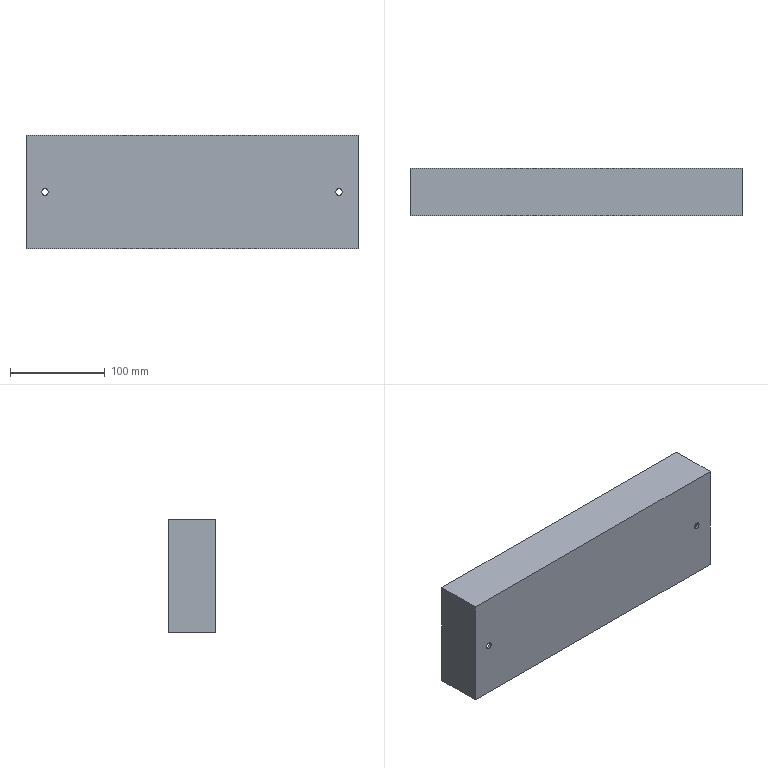Part | STEP file | J451-EBZ05-09-08-Part-1 | 1 solid | 15 faces | box 350 x 50 x 120 mm | volume 185346 mm3 | plane 11 | cylinder 4 | commonest cylinder face diameters 6.8 x4
STEP:
#1=CARTESIAN_POINT('',(0.,0.,0.));
#2=DIRECTION('',(0.,0.,1.));
#3=DIRECTION('',(1.,0.,0.));
#4=AXIS2_PLACEMENT_3D('',#1,#2,#3);
#5=CARTESIAN_POINT('',(16.6,2.3,60.));
#6=VERTEX_POINT('',#5);
#7=CARTESIAN_POINT('',(16.6,0.,60.));
#8=VERTEX_POINT('',#7);
#9=CARTESIAN_POINT('',(16.6,2.3,60.));
#10=DIRECTION('',(0.,-1.,0.));
#11=VECTOR('',#10,1.);
#12=LINE('',#9,#11);
#13=CARTESIAN_POINT('',(20.,2.3,60.));
#14=DIRECTION('',(0.,-1.,0.));
#15=DIRECTION('',(-1.,0.,0.));
#16=AXIS2_PLACEMENT_3D('',#13,#14,#15);
#17=CYLINDRICAL_SURFACE('',#16,3.4);
#18=CARTESIAN_POINT('',(6.283,0.));
#19=DIRECTION('',(0.,1.));
#20=VECTOR('',#19,1.);
#21=LINE('',#18,#20);
#22=(GEOMETRIC_REPRESENTATION_CONTEXT(2)PARAMETRIC_REPRESENTATION_CONTEXT()REPRESENTATION_CONTEXT('',''));
#23=DEFINITIONAL_REPRESENTATION('',(#21),#22);
#24=PCURVE('',#17,#23);
#25=CARTESIAN_POINT('',(20.,2.3,60.));
#26=DIRECTION('',(0.,-1.,0.));
#27=DIRECTION('',(-1.,0.,0.));
#28=AXIS2_PLACEMENT_3D('',#25,#26,#27);
#29=CYLINDRICAL_SURFACE('',#28,3.4);
#30=CARTESIAN_POINT('',(0.,0.));
#31=DIRECTION('',(0.,1.));
#32=VECTOR('',#31,1.);
#33=LINE('',#30,#32);
#34=(GEOMETRIC_REPRESENTATION_CONTEXT(2)PARAMETRIC_REPRESENTATION_CONTEXT()REPRESENTATION_CONTEXT('',''));
#35=DEFINITIONAL_REPRESENTATION('',(#33),#34);
#36=PCURVE('',#29,#35);
#37=SURFACE_CURVE('',#12,(#24,#36),.PCURVE_S1.);
#38=EDGE_CURVE('',#6,#8,#37,.T.);
#39=ORIENTED_EDGE('',*,*,#38,.T.);
#40=CARTESIAN_POINT('',(23.4,0.,60.));
#41=VERTEX_POINT('',#40);
#42=CARTESIAN_POINT('',(20.,0.,60.));
#43=DIRECTION('',(0.,1.,0.));
#44=DIRECTION('',(1.,0.,0.));
#45=AXIS2_PLACEMENT_3D('',#42,#43,#44);
#46=CIRCLE('',#45,3.4);
#47=CARTESIAN_POINT('',(9.425,2.3));
#48=DIRECTION('',(-1.,0.));
#49=VECTOR('',#48,1.);
#50=LINE('',#47,#49);
#51=(GEOMETRIC_REPRESENTATION_CONTEXT(2)PARAMETRIC_REPRESENTATION_CONTEXT()REPRESENTATION_CONTEXT('',''));
#52=DEFINITIONAL_REPRESENTATION('',(#50),#51);
#53=PCURVE('',#17,#52);
#54=CARTESIAN_POINT('',(2.,0.,60.));
#55=DIRECTION('',(0.,-1.,0.));
#56=DIRECTION('',(-1.,0.,0.));
#57=AXIS2_PLACEMENT_3D('',#54,#55,#56);
#58=PLANE('',#57);
#59=CARTESIAN_POINT('',(-21.4,0.));
#60=CARTESIAN_POINT('',(-21.4,5.889));
#61=CARTESIAN_POINT('',(-16.3,2.944));
#62=CARTESIAN_POINT('',(-11.2,0.));
#63=CARTESIAN_POINT('',(-16.3,-2.944));
#64=CARTESIAN_POINT('',(-21.4,-5.889));
#65=CARTESIAN_POINT('',(-21.4,0.));
#66=(BOUNDED_CURVE()B_SPLINE_CURVE(2,(#59,#60,#61,#62,#63,#64,#65),.UNSPECIFIED.,.T.,.F.)B_SPLINE_CURVE_WITH_KNOTS((1,2,2,2,2,1),(-2.094,0.,2.094,4.189,6.283,8.378),.UNSPECIFIED.)CURVE()GEOMETRIC_REPRESENTATION_ITEM()RATIONAL_B_SPLINE_CURVE((1.,0.5,1.,0.5,1.,0.5,1.))REPRESENTATION_ITEM(''));
#67=(GEOMETRIC_REPRESENTATION_CONTEXT(2)PARAMETRIC_REPRESENTATION_CONTEXT()REPRESENTATION_CONTEXT('',''));
#68=DEFINITIONAL_REPRESENTATION('',(#66),#67);
#69=PCURVE('',#58,#68);
#70=SURFACE_CURVE('',#46,(#53,#69),.PCURVE_S1.);
#71=EDGE_CURVE('',#8,#41,#70,.T.);
#72=ORIENTED_EDGE('',*,*,#71,.T.);
#73=CARTESIAN_POINT('',(23.4,2.3,60.));
#74=VERTEX_POINT('',#73);
#75=CARTESIAN_POINT('',(23.4,2.3,60.));
#76=DIRECTION('',(0.,-1.,0.));
#77=VECTOR('',#76,1.);
#78=LINE('',#75,#77);
#79=CARTESIAN_POINT('',(3.142,0.));
#80=DIRECTION('',(0.,1.));
#81=VECTOR('',#80,1.);
#82=LINE('',#79,#81);
#83=(GEOMETRIC_REPRESENTATION_CONTEXT(2)PARAMETRIC_REPRESENTATION_CONTEXT()REPRESENTATION_CONTEXT('',''));
#84=DEFINITIONAL_REPRESENTATION('',(#82),#83);
#85=PCURVE('',#17,#84);
#86=CARTESIAN_POINT('',(3.142,0.));
#87=DIRECTION('',(0.,1.));
#88=VECTOR('',#87,1.);
#89=LINE('',#86,#88);
#90=(GEOMETRIC_REPRESENTATION_CONTEXT(2)PARAMETRIC_REPRESENTATION_CONTEXT()REPRESENTATION_CONTEXT('',''));
#91=DEFINITIONAL_REPRESENTATION('',(#89),#90);
#92=PCURVE('',#29,#91);
#93=SURFACE_CURVE('',#78,(#85,#92),.PCURVE_S1.);
#94=EDGE_CURVE('',#74,#41,#93,.T.);
#95=ORIENTED_EDGE('',*,*,#94,.F.);
#96=CARTESIAN_POINT('',(20.,2.3,60.));
#97=DIRECTION('',(0.,-1.,0.));
#98=DIRECTION('',(-1.,0.,0.));
#99=AXIS2_PLACEMENT_3D('',#96,#97,#98);
#100=CIRCLE('',#99,3.4);
#101=CARTESIAN_POINT('',(0.,0.));
#102=DIRECTION('',(1.,0.));
#103=VECTOR('',#102,1.);
#104=LINE('',#101,#103);
#105=(GEOMETRIC_REPRESENTATION_CONTEXT(2)PARAMETRIC_REPRESENTATION_CONTEXT()REPRESENTATION_CONTEXT('',''));
#106=DEFINITIONAL_REPRESENTATION('',(#104),#105);
#107=PCURVE('',#17,#106);
#108=CARTESIAN_POINT('',(175.,2.3,60.));
#109=DIRECTION('',(0.,1.,0.));
#110=DIRECTION('',(0.,0.,1.));
#111=AXIS2_PLACEMENT_3D('',#108,#109,#110);
#112=PLANE('',#111);
#113=CARTESIAN_POINT('',(0.,-158.4));
#114=CARTESIAN_POINT('',(-5.889,-158.4));
#115=CARTESIAN_POINT('',(-2.944,-153.3));
#116=CARTESIAN_POINT('',(0.,-148.2));
#117=CARTESIAN_POINT('',(2.944,-153.3));
#118=CARTESIAN_POINT('',(5.889,-158.4));
#119=CARTESIAN_POINT('',(0.,-158.4));
#120=(BOUNDED_CURVE()B_SPLINE_CURVE(2,(#113,#114,#115,#116,#117,#118,#119),.UNSPECIFIED.,.T.,.F.)B_SPLINE_CURVE_WITH_KNOTS((1,2,2,2,2,1),(-2.094,0.,2.094,4.189,6.283,8.378),.UNSPECIFIED.)CURVE()GEOMETRIC_REPRESENTATION_ITEM()RATIONAL_B_SPLINE_CURVE((1.,0.5,1.,0.5,1.,0.5,1.))REPRESENTATION_ITEM(''));
#121=(GEOMETRIC_REPRESENTATION_CONTEXT(2)PARAMETRIC_REPRESENTATION_CONTEXT()REPRESENTATION_CONTEXT('',''));
#122=DEFINITIONAL_REPRESENTATION('',(#120),#121);
#123=PCURVE('',#112,#122);
#124=SURFACE_CURVE('',#100,(#107,#123),.PCURVE_S1.);
#125=EDGE_CURVE('',#74,#6,#124,.T.);
#126=ORIENTED_EDGE('',*,*,#125,.T.);
#127=EDGE_LOOP('',(#39,#72,#95,#126));
#128=FACE_BOUND('',#127,.F.);
#129=ADVANCED_FACE('',(#128),#17,.F.);
#130=CARTESIAN_POINT('',(326.6,2.3,60.));
#131=VERTEX_POINT('',#130);
#132=CARTESIAN_POINT('',(326.6,0.,60.));
#133=VERTEX_POINT('',#132);
#134=CARTESIAN_POINT('',(326.6,2.3,60.));
#135=DIRECTION('',(0.,-1.,0.));
#136=VECTOR('',#135,1.);
#137=LINE('',#134,#136);
#138=CARTESIAN_POINT('',(330.,2.3,60.));
#139=DIRECTION('',(0.,-1.,0.));
#140=DIRECTION('',(-1.,0.,0.));
#141=AXIS2_PLACEMENT_3D('',#138,#139,#140);
#142=CYLINDRICAL_SURFACE('',#141,3.4);
#143=CARTESIAN_POINT('',(6.283,0.));
#144=DIRECTION('',(0.,1.));
#145=VECTOR('',#144,1.);
#146=LINE('',#143,#145);
#147=(GEOMETRIC_REPRESENTATION_CONTEXT(2)PARAMETRIC_REPRESENTATION_CONTEXT()REPRESENTATION_CONTEXT('',''));
#148=DEFINITIONAL_REPRESENTATION('',(#146),#147);
#149=PCURVE('',#142,#148);
#150=CARTESIAN_POINT('',(330.,2.3,60.));
#151=DIRECTION('',(0.,-1.,0.));
#152=DIRECTION('',(-1.,0.,0.));
#153=AXIS2_PLACEMENT_3D('',#150,#151,#152);
#154=CYLINDRICAL_SURFACE('',#153,3.4);
#155=CARTESIAN_POINT('',(0.,0.));
#156=DIRECTION('',(0.,1.));
#157=VECTOR('',#156,1.);
#158=LINE('',#155,#157);
#159=(GEOMETRIC_REPRESENTATION_CONTEXT(2)PARAMETRIC_REPRESENTATION_CONTEXT()REPRESENTATION_CONTEXT('',''));
#160=DEFINITIONAL_REPRESENTATION('',(#158),#159);
#161=PCURVE('',#154,#160);
#162=SURFACE_CURVE('',#137,(#149,#161),.PCURVE_S1.);
#163=EDGE_CURVE('',#131,#133,#162,.T.);
#164=ORIENTED_EDGE('',*,*,#163,.T.);
#165=CARTESIAN_POINT('',(333.4,0.,60.));
#166=VERTEX_POINT('',#165);
#167=CARTESIAN_POINT('',(330.,0.,60.));
#168=DIRECTION('',(0.,1.,0.));
#169=DIRECTION('',(1.,0.,0.));
#170=AXIS2_PLACEMENT_3D('',#167,#168,#169);
#171=CIRCLE('',#170,3.4);
#172=CARTESIAN_POINT('',(9.425,2.3));
#173=DIRECTION('',(-1.,0.));
#174=VECTOR('',#173,1.);
#175=LINE('',#172,#174);
#176=(GEOMETRIC_REPRESENTATION_CONTEXT(2)PARAMETRIC_REPRESENTATION_CONTEXT()REPRESENTATION_CONTEXT('',''));
#177=DEFINITIONAL_REPRESENTATION('',(#175),#176);
#178=PCURVE('',#142,#177);
#179=CARTESIAN_POINT('',(-331.4,0.));
#180=CARTESIAN_POINT('',(-331.4,5.889));
#181=CARTESIAN_POINT('',(-326.3,2.944));
#182=CARTESIAN_POINT('',(-321.2,0.));
#183=CARTESIAN_POINT('',(-326.3,-2.944));
#184=CARTESIAN_POINT('',(-331.4,-5.889));
#185=CARTESIAN_POINT('',(-331.4,0.));
#186=(BOUNDED_CURVE()B_SPLINE_CURVE(2,(#179,#180,#181,#182,#183,#184,#185),.UNSPECIFIED.,.T.,.F.)B_SPLINE_CURVE_WITH_KNOTS((1,2,2,2,2,1),(-2.094,0.,2.094,4.189,6.283,8.378),.UNSPECIFIED.)CURVE()GEOMETRIC_REPRESENTATION_ITEM()RATIONAL_B_SPLINE_CURVE((1.,0.5,1.,0.5,1.,0.5,1.))REPRESENTATION_ITEM(''));
#187=(GEOMETRIC_REPRESENTATION_CONTEXT(2)PARAMETRIC_REPRESENTATION_CONTEXT()REPRESENTATION_CONTEXT('',''));
#188=DEFINITIONAL_REPRESENTATION('',(#186),#187);
#189=PCURVE('',#58,#188);
#190=SURFACE_CURVE('',#171,(#178,#189),.PCURVE_S1.);
#191=EDGE_CURVE('',#133,#166,#190,.T.);
#192=ORIENTED_EDGE('',*,*,#191,.T.);
#193=CARTESIAN_POINT('',(333.4,2.3,60.));
#194=VERTEX_POINT('',#193);
#195=CARTESIAN_POINT('',(333.4,2.3,60.));
#196=DIRECTION('',(0.,-1.,0.));
#197=VECTOR('',#196,1.);
#198=LINE('',#195,#197);
#199=CARTESIAN_POINT('',(3.142,0.));
#200=DIRECTION('',(0.,1.));
#201=VECTOR('',#200,1.);
#202=LINE('',#199,#201);
#203=(GEOMETRIC_REPRESENTATION_CONTEXT(2)PARAMETRIC_REPRESENTATION_CONTEXT()REPRESENTATION_CONTEXT('',''));
#204=DEFINITIONAL_REPRESENTATION('',(#202),#203);
#205=PCURVE('',#142,#204);
#206=CARTESIAN_POINT('',(3.142,0.));
#207=DIRECTION('',(0.,1.));
#208=VECTOR('',#207,1.);
#209=LINE('',#206,#208);
#210=(GEOMETRIC_REPRESENTATION_CONTEXT(2)PARAMETRIC_REPRESENTATION_CONTEXT()REPRESENTATION_CONTEXT('',''));
#211=DEFINITIONAL_REPRESENTATION('',(#209),#210);
#212=PCURVE('',#154,#211);
#213=SURFACE_CURVE('',#198,(#205,#212),.PCURVE_S1.);
#214=EDGE_CURVE('',#194,#166,#213,.T.);
#215=ORIENTED_EDGE('',*,*,#214,.F.);
#216=CARTESIAN_POINT('',(330.,2.3,60.));
#217=DIRECTION('',(0.,-1.,0.));
#218=DIRECTION('',(-1.,0.,0.));
#219=AXIS2_PLACEMENT_3D('',#216,#217,#218);
#220=CIRCLE('',#219,3.4);
#221=CARTESIAN_POINT('',(0.,0.));
#222=DIRECTION('',(1.,0.));
#223=VECTOR('',#222,1.);
#224=LINE('',#221,#223);
#225=(GEOMETRIC_REPRESENTATION_CONTEXT(2)PARAMETRIC_REPRESENTATION_CONTEXT()REPRESENTATION_CONTEXT('',''));
#226=DEFINITIONAL_REPRESENTATION('',(#224),#225);
#227=PCURVE('',#142,#226);
#228=CARTESIAN_POINT('',(0.,151.6));
#229=CARTESIAN_POINT('',(-5.889,151.6));
#230=CARTESIAN_POINT('',(-2.944,156.7));
#231=CARTESIAN_POINT('',(0.,161.8));
#232=CARTESIAN_POINT('',(2.944,156.7));
#233=CARTESIAN_POINT('',(5.889,151.6));
#234=CARTESIAN_POINT('',(0.,151.6));
#235=(BOUNDED_CURVE()B_SPLINE_CURVE(2,(#228,#229,#230,#231,#232,#233,#234),.UNSPECIFIED.,.T.,.F.)B_SPLINE_CURVE_WITH_KNOTS((1,2,2,2,2,1),(-2.094,0.,2.094,4.189,6.283,8.378),.UNSPECIFIED.)CURVE()GEOMETRIC_REPRESENTATION_ITEM()RATIONAL_B_SPLINE_CURVE((1.,0.5,1.,0.5,1.,0.5,1.))REPRESENTATION_ITEM(''));
#236=(GEOMETRIC_REPRESENTATION_CONTEXT(2)PARAMETRIC_REPRESENTATION_CONTEXT()REPRESENTATION_CONTEXT('',''));
#237=DEFINITIONAL_REPRESENTATION('',(#235),#236);
#238=PCURVE('',#112,#237);
#239=SURFACE_CURVE('',#220,(#227,#238),.PCURVE_S1.);
#240=EDGE_CURVE('',#194,#131,#239,.T.);
#241=ORIENTED_EDGE('',*,*,#240,.T.);
#242=EDGE_LOOP('',(#164,#192,#215,#241));
#243=FACE_BOUND('',#242,.F.);
#244=ADVANCED_FACE('',(#243),#142,.F.);
#245=CARTESIAN_POINT('',(0.,50.,120.));
#246=VERTEX_POINT('',#245);
#247=CARTESIAN_POINT('',(0.,0.,120.));
#248=VERTEX_POINT('',#247);
#249=CARTESIAN_POINT('',(0.,25.,120.));
#250=DIRECTION('',(0.,-1.,0.));
#251=VECTOR('',#250,1.);
#252=LINE('',#249,#251);
#253=CARTESIAN_POINT('',(0.,25.,60.));
#254=DIRECTION('',(-1.,0.,0.));
#255=DIRECTION('',(0.,1.,0.));
#256=AXIS2_PLACEMENT_3D('',#253,#254,#255);
#257=PLANE('',#256);
#258=CARTESIAN_POINT('',(0.,-60.));
#259=DIRECTION('',(-1.,0.));
#260=VECTOR('',#259,1.);
#261=LINE('',#258,#260);
#262=(GEOMETRIC_REPRESENTATION_CONTEXT(2)PARAMETRIC_REPRESENTATION_CONTEXT()REPRESENTATION_CONTEXT('',''));
#263=DEFINITIONAL_REPRESENTATION('',(#261),#262);
#264=PCURVE('',#257,#263);
#265=CARTESIAN_POINT('',(2.,25.,120.));
#266=DIRECTION('',(0.,0.,1.));
#267=DIRECTION('',(1.,0.,0.));
#268=AXIS2_PLACEMENT_3D('',#265,#266,#267);
#269=PLANE('',#268);
#270=CARTESIAN_POINT('',(-2.,0.));
#271=DIRECTION('',(0.,-1.));
#272=VECTOR('',#271,1.);
#273=LINE('',#270,#272);
#274=(GEOMETRIC_REPRESENTATION_CONTEXT(2)PARAMETRIC_REPRESENTATION_CONTEXT()REPRESENTATION_CONTEXT('',''));
#275=DEFINITIONAL_REPRESENTATION('',(#273),#274);
#276=PCURVE('',#269,#275);
#277=SURFACE_CURVE('',#252,(#264,#276),.PCURVE_S1.);
#278=EDGE_CURVE('',#246,#248,#277,.T.);
#279=ORIENTED_EDGE('',*,*,#278,.F.);
#280=CARTESIAN_POINT('',(0.,50.,0.));
#281=VERTEX_POINT('',#280);
#282=CARTESIAN_POINT('',(0.,50.,60.));
#283=DIRECTION('',(0.,0.,1.));
#284=VECTOR('',#283,1.);
#285=LINE('',#282,#284);
#286=CARTESIAN_POINT('',(25.,0.));
#287=DIRECTION('',(0.,-1.));
#288=VECTOR('',#287,1.);
#289=LINE('',#286,#288);
#290=(GEOMETRIC_REPRESENTATION_CONTEXT(2)PARAMETRIC_REPRESENTATION_CONTEXT()REPRESENTATION_CONTEXT('',''));
#291=DEFINITIONAL_REPRESENTATION('',(#289),#290);
#292=PCURVE('',#257,#291);
#293=CARTESIAN_POINT('',(2.,50.,60.));
#294=DIRECTION('',(0.,1.,0.));
#295=DIRECTION('',(1.,0.,0.));
#296=AXIS2_PLACEMENT_3D('',#293,#294,#295);
#297=PLANE('',#296);
#298=CARTESIAN_POINT('',(-2.,0.));
#299=DIRECTION('',(0.,-1.));
#300=VECTOR('',#299,1.);
#301=LINE('',#298,#300);
#302=(GEOMETRIC_REPRESENTATION_CONTEXT(2)PARAMETRIC_REPRESENTATION_CONTEXT()REPRESENTATION_CONTEXT('',''));
#303=DEFINITIONAL_REPRESENTATION('',(#301),#302);
#304=PCURVE('',#297,#303);
#305=SURFACE_CURVE('',#285,(#292,#304),.PCURVE_S1.);
#306=EDGE_CURVE('',#281,#246,#305,.T.);
#307=ORIENTED_EDGE('',*,*,#306,.F.);
#308=CARTESIAN_POINT('',(0.,0.,0.));
#309=VERTEX_POINT('',#308);
#310=CARTESIAN_POINT('',(0.,25.,0.));
#311=DIRECTION('',(0.,1.,0.));
#312=VECTOR('',#311,1.);
#313=LINE('',#310,#312);
#314=CARTESIAN_POINT('',(0.,60.));
#315=DIRECTION('',(1.,0.));
#316=VECTOR('',#315,1.);
#317=LINE('',#314,#316);
#318=(GEOMETRIC_REPRESENTATION_CONTEXT(2)PARAMETRIC_REPRESENTATION_CONTEXT()REPRESENTATION_CONTEXT('',''));
#319=DEFINITIONAL_REPRESENTATION('',(#317),#318);
#320=PCURVE('',#257,#319);
#321=CARTESIAN_POINT('',(2.,25.,0.));
#322=DIRECTION('',(0.,0.,-1.));
#323=DIRECTION('',(-1.,0.,0.));
#324=AXIS2_PLACEMENT_3D('',#321,#322,#323);
#325=PLANE('',#324);
#326=CARTESIAN_POINT('',(2.,0.));
#327=DIRECTION('',(0.,1.));
#328=VECTOR('',#327,1.);
#329=LINE('',#326,#328);
#330=(GEOMETRIC_REPRESENTATION_CONTEXT(2)PARAMETRIC_REPRESENTATION_CONTEXT()REPRESENTATION_CONTEXT('',''));
#331=DEFINITIONAL_REPRESENTATION('',(#329),#330);
#332=PCURVE('',#325,#331);
#333=SURFACE_CURVE('',#313,(#320,#332),.PCURVE_S1.);
#334=EDGE_CURVE('',#309,#281,#333,.T.);
#335=ORIENTED_EDGE('',*,*,#334,.F.);
#336=CARTESIAN_POINT('',(0.,0.,60.));
#337=DIRECTION('',(0.,0.,-1.));
#338=VECTOR('',#337,1.);
#339=LINE('',#336,#338);
#340=CARTESIAN_POINT('',(-25.,0.));
#341=DIRECTION('',(0.,1.));
#342=VECTOR('',#341,1.);
#343=LINE('',#340,#342);
#344=(GEOMETRIC_REPRESENTATION_CONTEXT(2)PARAMETRIC_REPRESENTATION_CONTEXT()REPRESENTATION_CONTEXT('',''));
#345=DEFINITIONAL_REPRESENTATION('',(#343),#344);
#346=PCURVE('',#257,#345);
#347=CARTESIAN_POINT('',(2.,0.));
#348=DIRECTION('',(0.,1.));
#349=VECTOR('',#348,1.);
#350=LINE('',#347,#349);
#351=(GEOMETRIC_REPRESENTATION_CONTEXT(2)PARAMETRIC_REPRESENTATION_CONTEXT()REPRESENTATION_CONTEXT('',''));
#352=DEFINITIONAL_REPRESENTATION('',(#350),#351);
#353=PCURVE('',#58,#352);
#354=SURFACE_CURVE('',#339,(#346,#353),.PCURVE_S1.);
#355=EDGE_CURVE('',#248,#309,#354,.T.);
#356=ORIENTED_EDGE('',*,*,#355,.F.);
#357=EDGE_LOOP('',(#279,#307,#335,#356));
#358=FACE_BOUND('',#357,.T.);
#359=ADVANCED_FACE('',(#358),#257,.T.);
#360=ORIENTED_EDGE('',*,*,#278,.T.);
#361=CARTESIAN_POINT('',(350.,0.,120.));
#362=VERTEX_POINT('',#361);
#363=CARTESIAN_POINT('',(2.,0.,120.));
#364=DIRECTION('',(-1.,0.,0.));
#365=VECTOR('',#364,1.);
#366=LINE('',#363,#365);
#367=CARTESIAN_POINT('',(0.,-25.));
#368=DIRECTION('',(-1.,0.));
#369=VECTOR('',#368,1.);
#370=LINE('',#367,#369);
#371=(GEOMETRIC_REPRESENTATION_CONTEXT(2)PARAMETRIC_REPRESENTATION_CONTEXT()REPRESENTATION_CONTEXT('',''));
#372=DEFINITIONAL_REPRESENTATION('',(#370),#371);
#373=PCURVE('',#269,#372);
#374=CARTESIAN_POINT('',(0.,-60.));
#375=DIRECTION('',(1.,0.));
#376=VECTOR('',#375,1.);
#377=LINE('',#374,#376);
#378=(GEOMETRIC_REPRESENTATION_CONTEXT(2)PARAMETRIC_REPRESENTATION_CONTEXT()REPRESENTATION_CONTEXT('',''));
#379=DEFINITIONAL_REPRESENTATION('',(#377),#378);
#380=PCURVE('',#58,#379);
#381=SURFACE_CURVE('',#366,(#373,#380),.PCURVE_S1.);
#382=EDGE_CURVE('',#362,#248,#381,.T.);
#383=ORIENTED_EDGE('',*,*,#382,.F.);
#384=CARTESIAN_POINT('',(350.,50.,120.));
#385=VERTEX_POINT('',#384);
#386=CARTESIAN_POINT('',(350.,25.,120.));
#387=DIRECTION('',(0.,-1.,0.));
#388=VECTOR('',#387,1.);
#389=LINE('',#386,#388);
#390=CARTESIAN_POINT('',(348.,0.));
#391=DIRECTION('',(0.,-1.));
#392=VECTOR('',#391,1.);
#393=LINE('',#390,#392);
#394=(GEOMETRIC_REPRESENTATION_CONTEXT(2)PARAMETRIC_REPRESENTATION_CONTEXT()REPRESENTATION_CONTEXT('',''));
#395=DEFINITIONAL_REPRESENTATION('',(#393),#394);
#396=PCURVE('',#269,#395);
#397=CARTESIAN_POINT('',(350.,25.,120.));
#398=DIRECTION('',(1.,0.,0.));
#399=DIRECTION('',(0.,0.,-1.));
#400=AXIS2_PLACEMENT_3D('',#397,#398,#399);
#401=PLANE('',#400);
#402=CARTESIAN_POINT('',(0.,0.));
#403=DIRECTION('',(0.,-1.));
#404=VECTOR('',#403,1.);
#405=LINE('',#402,#404);
#406=(GEOMETRIC_REPRESENTATION_CONTEXT(2)PARAMETRIC_REPRESENTATION_CONTEXT()REPRESENTATION_CONTEXT('',''));
#407=DEFINITIONAL_REPRESENTATION('',(#405),#406);
#408=PCURVE('',#401,#407);
#409=SURFACE_CURVE('',#389,(#396,#408),.PCURVE_S1.);
#410=EDGE_CURVE('',#385,#362,#409,.T.);
#411=ORIENTED_EDGE('',*,*,#410,.F.);
#412=CARTESIAN_POINT('',(2.,50.,120.));
#413=DIRECTION('',(-1.,0.,0.));
#414=VECTOR('',#413,1.);
#415=LINE('',#412,#414);
#416=CARTESIAN_POINT('',(0.,25.));
#417=DIRECTION('',(-1.,0.));
#418=VECTOR('',#417,1.);
#419=LINE('',#416,#418);
#420=(GEOMETRIC_REPRESENTATION_CONTEXT(2)PARAMETRIC_REPRESENTATION_CONTEXT()REPRESENTATION_CONTEXT('',''));
#421=DEFINITIONAL_REPRESENTATION('',(#419),#420);
#422=PCURVE('',#269,#421);
#423=CARTESIAN_POINT('',(0.,-60.));
#424=DIRECTION('',(-1.,0.));
#425=VECTOR('',#424,1.);
#426=LINE('',#423,#425);
#427=(GEOMETRIC_REPRESENTATION_CONTEXT(2)PARAMETRIC_REPRESENTATION_CONTEXT()REPRESENTATION_CONTEXT('',''));
#428=DEFINITIONAL_REPRESENTATION('',(#426),#427);
#429=PCURVE('',#297,#428);
#430=SURFACE_CURVE('',#415,(#422,#429),.PCURVE_S1.);
#431=EDGE_CURVE('',#385,#246,#430,.T.);
#432=ORIENTED_EDGE('',*,*,#431,.T.);
#433=EDGE_LOOP('',(#360,#383,#411,#432));
#434=FACE_BOUND('',#433,.T.);
#435=ADVANCED_FACE('',(#434),#269,.T.);
#436=ORIENTED_EDGE('',*,*,#71,.T.);
#437=CARTESIAN_POINT('',(20.,0.,60.));
#438=DIRECTION('',(0.,1.,0.));
#439=DIRECTION('',(1.,0.,0.));
#440=AXIS2_PLACEMENT_3D('',#437,#438,#439);
#441=CIRCLE('',#440,3.4);
#442=CARTESIAN_POINT('',(-21.4,0.));
#443=CARTESIAN_POINT('',(-21.4,5.889));
#444=CARTESIAN_POINT('',(-16.3,2.944));
#445=CARTESIAN_POINT('',(-11.2,0.));
#446=CARTESIAN_POINT('',(-16.3,-2.944));
#447=CARTESIAN_POINT('',(-21.4,-5.889));
#448=CARTESIAN_POINT('',(-21.4,0.));
#449=(BOUNDED_CURVE()B_SPLINE_CURVE(2,(#442,#443,#444,#445,#446,#447,#448),.UNSPECIFIED.,.T.,.F.)B_SPLINE_CURVE_WITH_KNOTS((1,2,2,2,2,1),(-2.094,0.,2.094,4.189,6.283,8.378),.UNSPECIFIED.)CURVE()GEOMETRIC_REPRESENTATION_ITEM()RATIONAL_B_SPLINE_CURVE((1.,0.5,1.,0.5,1.,0.5,1.))REPRESENTATION_ITEM(''));
#450=(GEOMETRIC_REPRESENTATION_CONTEXT(2)PARAMETRIC_REPRESENTATION_CONTEXT()REPRESENTATION_CONTEXT('',''));
#451=DEFINITIONAL_REPRESENTATION('',(#449),#450);
#452=PCURVE('',#58,#451);
#453=CARTESIAN_POINT('',(3.142,2.3));
#454=DIRECTION('',(-1.,0.));
#455=VECTOR('',#454,1.);
#456=LINE('',#453,#455);
#457=(GEOMETRIC_REPRESENTATION_CONTEXT(2)PARAMETRIC_REPRESENTATION_CONTEXT()REPRESENTATION_CONTEXT('',''));
#458=DEFINITIONAL_REPRESENTATION('',(#456),#457);
#459=PCURVE('',#29,#458);
#460=SURFACE_CURVE('',#441,(#452,#459),.PCURVE_S1.);
#461=EDGE_CURVE('',#41,#8,#460,.T.);
#462=ORIENTED_EDGE('',*,*,#461,.T.);
#463=EDGE_LOOP('',(#436,#462));
#464=FACE_BOUND('',#463,.T.);
#465=ORIENTED_EDGE('',*,*,#191,.T.);
#466=CARTESIAN_POINT('',(330.,0.,60.));
#467=DIRECTION('',(0.,1.,0.));
#468=DIRECTION('',(1.,0.,0.));
#469=AXIS2_PLACEMENT_3D('',#466,#467,#468);
#470=CIRCLE('',#469,3.4);
#471=CARTESIAN_POINT('',(-331.4,0.));
#472=CARTESIAN_POINT('',(-331.4,5.889));
#473=CARTESIAN_POINT('',(-326.3,2.944));
#474=CARTESIAN_POINT('',(-321.2,0.));
#475=CARTESIAN_POINT('',(-326.3,-2.944));
#476=CARTESIAN_POINT('',(-331.4,-5.889));
#477=CARTESIAN_POINT('',(-331.4,0.));
#478=(BOUNDED_CURVE()B_SPLINE_CURVE(2,(#471,#472,#473,#474,#475,#476,#477),.UNSPECIFIED.,.T.,.F.)B_SPLINE_CURVE_WITH_KNOTS((1,2,2,2,2,1),(-2.094,0.,2.094,4.189,6.283,8.378),.UNSPECIFIED.)CURVE()GEOMETRIC_REPRESENTATION_ITEM()RATIONAL_B_SPLINE_CURVE((1.,0.5,1.,0.5,1.,0.5,1.))REPRESENTATION_ITEM(''));
#479=(GEOMETRIC_REPRESENTATION_CONTEXT(2)PARAMETRIC_REPRESENTATION_CONTEXT()REPRESENTATION_CONTEXT('',''));
#480=DEFINITIONAL_REPRESENTATION('',(#478),#479);
#481=PCURVE('',#58,#480);
#482=CARTESIAN_POINT('',(3.142,2.3));
#483=DIRECTION('',(-1.,0.));
#484=VECTOR('',#483,1.);
#485=LINE('',#482,#484);
#486=(GEOMETRIC_REPRESENTATION_CONTEXT(2)PARAMETRIC_REPRESENTATION_CONTEXT()REPRESENTATION_CONTEXT('',''));
#487=DEFINITIONAL_REPRESENTATION('',(#485),#486);
#488=PCURVE('',#154,#487);
#489=SURFACE_CURVE('',#470,(#481,#488),.PCURVE_S1.);
#490=EDGE_CURVE('',#166,#133,#489,.T.);
#491=ORIENTED_EDGE('',*,*,#490,.T.);
#492=EDGE_LOOP('',(#465,#491));
#493=FACE_BOUND('',#492,.T.);
#494=CARTESIAN_POINT('',(350.,0.,0.));
#495=VERTEX_POINT('',#494);
#496=CARTESIAN_POINT('',(2.,0.,0.));
#497=DIRECTION('',(-1.,0.,0.));
#498=VECTOR('',#497,1.);
#499=LINE('',#496,#498);
#500=CARTESIAN_POINT('',(0.,60.));
#501=DIRECTION('',(1.,0.));
#502=VECTOR('',#501,1.);
#503=LINE('',#500,#502);
#504=(GEOMETRIC_REPRESENTATION_CONTEXT(2)PARAMETRIC_REPRESENTATION_CONTEXT()REPRESENTATION_CONTEXT('',''));
#505=DEFINITIONAL_REPRESENTATION('',(#503),#504);
#506=PCURVE('',#58,#505);
#507=CARTESIAN_POINT('',(0.,-25.));
#508=DIRECTION('',(1.,0.));
#509=VECTOR('',#508,1.);
#510=LINE('',#507,#509);
#511=(GEOMETRIC_REPRESENTATION_CONTEXT(2)PARAMETRIC_REPRESENTATION_CONTEXT()REPRESENTATION_CONTEXT('',''));
#512=DEFINITIONAL_REPRESENTATION('',(#510),#511);
#513=PCURVE('',#325,#512);
#514=SURFACE_CURVE('',#499,(#506,#513),.PCURVE_S1.);
#515=EDGE_CURVE('',#495,#309,#514,.T.);
#516=ORIENTED_EDGE('',*,*,#515,.F.);
#517=CARTESIAN_POINT('',(350.,0.,120.));
#518=DIRECTION('',(0.,0.,-1.));
#519=VECTOR('',#518,1.);
#520=LINE('',#517,#519);
#521=CARTESIAN_POINT('',(-348.,-60.));
#522=DIRECTION('',(0.,1.));
#523=VECTOR('',#522,1.);
#524=LINE('',#521,#523);
#525=(GEOMETRIC_REPRESENTATION_CONTEXT(2)PARAMETRIC_REPRESENTATION_CONTEXT()REPRESENTATION_CONTEXT('',''));
#526=DEFINITIONAL_REPRESENTATION('',(#524),#525);
#527=PCURVE('',#58,#526);
#528=CARTESIAN_POINT('',(0.,-25.));
#529=DIRECTION('',(1.,0.));
#530=VECTOR('',#529,1.);
#531=LINE('',#528,#530);
#532=(GEOMETRIC_REPRESENTATION_CONTEXT(2)PARAMETRIC_REPRESENTATION_CONTEXT()REPRESENTATION_CONTEXT('',''));
#533=DEFINITIONAL_REPRESENTATION('',(#531),#532);
#534=PCURVE('',#401,#533);
#535=SURFACE_CURVE('',#520,(#527,#534),.PCURVE_S1.);
#536=EDGE_CURVE('',#362,#495,#535,.T.);
#537=ORIENTED_EDGE('',*,*,#536,.F.);
#538=ORIENTED_EDGE('',*,*,#382,.T.);
#539=ORIENTED_EDGE('',*,*,#355,.T.);
#540=EDGE_LOOP('',(#516,#537,#538,#539));
#541=FACE_BOUND('',#540,.T.);
#542=ADVANCED_FACE('',(#464,#493,#541),#58,.T.);
#543=CARTESIAN_POINT('',(350.,50.,0.));
#544=VERTEX_POINT('',#543);
#545=CARTESIAN_POINT('',(2.,50.,0.));
#546=DIRECTION('',(-1.,0.,0.));
#547=VECTOR('',#546,1.);
#548=LINE('',#545,#547);
#549=CARTESIAN_POINT('',(0.,25.));
#550=DIRECTION('',(1.,0.));
#551=VECTOR('',#550,1.);
#552=LINE('',#549,#551);
#553=(GEOMETRIC_REPRESENTATION_CONTEXT(2)PARAMETRIC_REPRESENTATION_CONTEXT()REPRESENTATION_CONTEXT('',''));
#554=DEFINITIONAL_REPRESENTATION('',(#552),#553);
#555=PCURVE('',#325,#554);
#556=CARTESIAN_POINT('',(0.,60.));
#557=DIRECTION('',(-1.,0.));
#558=VECTOR('',#557,1.);
#559=LINE('',#556,#558);
#560=(GEOMETRIC_REPRESENTATION_CONTEXT(2)PARAMETRIC_REPRESENTATION_CONTEXT()REPRESENTATION_CONTEXT('',''));
#561=DEFINITIONAL_REPRESENTATION('',(#559),#560);
#562=PCURVE('',#297,#561);
#563=SURFACE_CURVE('',#548,(#555,#562),.PCURVE_S1.);
#564=EDGE_CURVE('',#544,#281,#563,.T.);
#565=ORIENTED_EDGE('',*,*,#564,.F.);
#566=CARTESIAN_POINT('',(350.,25.,0.));
#567=DIRECTION('',(0.,-1.,0.));
#568=VECTOR('',#567,1.);
#569=LINE('',#566,#568);
#570=CARTESIAN_POINT('',(-348.,0.));
#571=DIRECTION('',(0.,-1.));
#572=VECTOR('',#571,1.);
#573=LINE('',#570,#572);
#574=(GEOMETRIC_REPRESENTATION_CONTEXT(2)PARAMETRIC_REPRESENTATION_CONTEXT()REPRESENTATION_CONTEXT('',''));
#575=DEFINITIONAL_REPRESENTATION('',(#573),#574);
#576=PCURVE('',#325,#575);
#577=CARTESIAN_POINT('',(120.,0.));
#578=DIRECTION('',(0.,-1.));
#579=VECTOR('',#578,1.);
#580=LINE('',#577,#579);
#581=(GEOMETRIC_REPRESENTATION_CONTEXT(2)PARAMETRIC_REPRESENTATION_CONTEXT()REPRESENTATION_CONTEXT('',''));
#582=DEFINITIONAL_REPRESENTATION('',(#580),#581);
#583=PCURVE('',#401,#582);
#584=SURFACE_CURVE('',#569,(#576,#583),.PCURVE_S1.);
#585=EDGE_CURVE('',#544,#495,#584,.T.);
#586=ORIENTED_EDGE('',*,*,#585,.T.);
#587=ORIENTED_EDGE('',*,*,#515,.T.);
#588=ORIENTED_EDGE('',*,*,#334,.T.);
#589=EDGE_LOOP('',(#565,#586,#587,#588));
#590=FACE_BOUND('',#589,.T.);
#591=ADVANCED_FACE('',(#590),#325,.T.);
#592=CARTESIAN_POINT('',(2.,2.3,118.));
#593=VERTEX_POINT('',#592);
#594=CARTESIAN_POINT('',(2.,50.,118.));
#595=VERTEX_POINT('',#594);
#596=CARTESIAN_POINT('',(2.,25.,118.));
#597=DIRECTION('',(0.,1.,0.));
#598=VECTOR('',#597,1.);
#599=LINE('',#596,#598);
#600=CARTESIAN_POINT('',(2.,25.,60.));
#601=DIRECTION('',(1.,0.,0.));
#602=DIRECTION('',(0.,-1.,0.));
#603=AXIS2_PLACEMENT_3D('',#600,#601,#602);
#604=PLANE('',#603);
#605=CARTESIAN_POINT('',(0.,-58.));
#606=DIRECTION('',(-1.,0.));
#607=VECTOR('',#606,1.);
#608=LINE('',#605,#607);
#609=(GEOMETRIC_REPRESENTATION_CONTEXT(2)PARAMETRIC_REPRESENTATION_CONTEXT()REPRESENTATION_CONTEXT('',''));
#610=DEFINITIONAL_REPRESENTATION('',(#608),#609);
#611=PCURVE('',#604,#610);
#612=CARTESIAN_POINT('',(175.,25.,118.));
#613=DIRECTION('',(0.,0.,-1.));
#614=DIRECTION('',(0.,1.,0.));
#615=AXIS2_PLACEMENT_3D('',#612,#613,#614);
#616=PLANE('',#615);
#617=CARTESIAN_POINT('',(0.,-173.));
#618=DIRECTION('',(1.,0.));
#619=VECTOR('',#618,1.);
#620=LINE('',#617,#619);
#621=(GEOMETRIC_REPRESENTATION_CONTEXT(2)PARAMETRIC_REPRESENTATION_CONTEXT()REPRESENTATION_CONTEXT('',''));
#622=DEFINITIONAL_REPRESENTATION('',(#620),#621);
#623=PCURVE('',#616,#622);
#624=SURFACE_CURVE('',#599,(#611,#623),.PCURVE_S1.);
#625=EDGE_CURVE('',#593,#595,#624,.T.);
#626=ORIENTED_EDGE('',*,*,#625,.F.);
#627=CARTESIAN_POINT('',(2.,2.3,2.));
#628=VERTEX_POINT('',#627);
#629=CARTESIAN_POINT('',(2.,2.3,60.));
#630=DIRECTION('',(0.,0.,1.));
#631=VECTOR('',#630,1.);
#632=LINE('',#629,#631);
#633=CARTESIAN_POINT('',(22.7,0.));
#634=DIRECTION('',(0.,-1.));
#635=VECTOR('',#634,1.);
#636=LINE('',#633,#635);
#637=(GEOMETRIC_REPRESENTATION_CONTEXT(2)PARAMETRIC_REPRESENTATION_CONTEXT()REPRESENTATION_CONTEXT('',''));
#638=DEFINITIONAL_REPRESENTATION('',(#636),#637);
#639=PCURVE('',#604,#638);
#640=CARTESIAN_POINT('',(0.,-173.));
#641=DIRECTION('',(1.,0.));
#642=VECTOR('',#641,1.);
#643=LINE('',#640,#642);
#644=(GEOMETRIC_REPRESENTATION_CONTEXT(2)PARAMETRIC_REPRESENTATION_CONTEXT()REPRESENTATION_CONTEXT('',''));
#645=DEFINITIONAL_REPRESENTATION('',(#643),#644);
#646=PCURVE('',#112,#645);
#647=SURFACE_CURVE('',#632,(#639,#646),.PCURVE_S1.);
#648=EDGE_CURVE('',#628,#593,#647,.T.);
#649=ORIENTED_EDGE('',*,*,#648,.F.);
#650=CARTESIAN_POINT('',(2.,50.,2.));
#651=VERTEX_POINT('',#650);
#652=CARTESIAN_POINT('',(2.,25.,2.));
#653=DIRECTION('',(0.,-1.,0.));
#654=VECTOR('',#653,1.);
#655=LINE('',#652,#654);
#656=CARTESIAN_POINT('',(0.,58.));
#657=DIRECTION('',(1.,0.));
#658=VECTOR('',#657,1.);
#659=LINE('',#656,#658);
#660=(GEOMETRIC_REPRESENTATION_CONTEXT(2)PARAMETRIC_REPRESENTATION_CONTEXT()REPRESENTATION_CONTEXT('',''));
#661=DEFINITIONAL_REPRESENTATION('',(#659),#660);
#662=PCURVE('',#604,#661);
#663=CARTESIAN_POINT('',(175.,25.,2.));
#664=DIRECTION('',(0.,0.,1.));
#665=DIRECTION('',(0.,-1.,0.));
#666=AXIS2_PLACEMENT_3D('',#663,#664,#665);
#667=PLANE('',#666);
#668=CARTESIAN_POINT('',(0.,-173.));
#669=DIRECTION('',(1.,0.));
#670=VECTOR('',#669,1.);
#671=LINE('',#668,#670);
#672=(GEOMETRIC_REPRESENTATION_CONTEXT(2)PARAMETRIC_REPRESENTATION_CONTEXT()REPRESENTATION_CONTEXT('',''));
#673=DEFINITIONAL_REPRESENTATION('',(#671),#672);
#674=PCURVE('',#667,#673);
#675=SURFACE_CURVE('',#655,(#662,#674),.PCURVE_S1.);
#676=EDGE_CURVE('',#651,#628,#675,.T.);
#677=ORIENTED_EDGE('',*,*,#676,.F.);
#678=CARTESIAN_POINT('',(2.,50.,60.));
#679=DIRECTION('',(0.,0.,-1.));
#680=VECTOR('',#679,1.);
#681=LINE('',#678,#680);
#682=CARTESIAN_POINT('',(-25.,0.));
#683=DIRECTION('',(0.,1.));
#684=VECTOR('',#683,1.);
#685=LINE('',#682,#684);
#686=(GEOMETRIC_REPRESENTATION_CONTEXT(2)PARAMETRIC_REPRESENTATION_CONTEXT()REPRESENTATION_CONTEXT('',''));
#687=DEFINITIONAL_REPRESENTATION('',(#685),#686);
#688=PCURVE('',#604,#687);
#689=CARTESIAN_POINT('',(0.,0.));
#690=DIRECTION('',(0.,1.));
#691=VECTOR('',#690,1.);
#692=LINE('',#689,#691);
#693=(GEOMETRIC_REPRESENTATION_CONTEXT(2)PARAMETRIC_REPRESENTATION_CONTEXT()REPRESENTATION_CONTEXT('',''));
#694=DEFINITIONAL_REPRESENTATION('',(#692),#693);
#695=PCURVE('',#297,#694);
#696=SURFACE_CURVE('',#681,(#688,#695),.PCURVE_S1.);
#697=EDGE_CURVE('',#595,#651,#696,.T.);
#698=ORIENTED_EDGE('',*,*,#697,.F.);
#699=EDGE_LOOP('',(#626,#649,#677,#698));
#700=FACE_BOUND('',#699,.T.);
#701=ADVANCED_FACE('',(#700),#604,.T.);
#702=CARTESIAN_POINT('',(348.,50.,2.));
#703=VERTEX_POINT('',#702);
#704=CARTESIAN_POINT('',(175.,50.,2.));
#705=DIRECTION('',(1.,0.,0.));
#706=VECTOR('',#705,1.);
#707=LINE('',#704,#706);
#708=CARTESIAN_POINT('',(173.,58.));
#709=DIRECTION('',(1.,0.));
#710=VECTOR('',#709,1.);
#711=LINE('',#708,#710);
#712=(GEOMETRIC_REPRESENTATION_CONTEXT(2)PARAMETRIC_REPRESENTATION_CONTEXT()REPRESENTATION_CONTEXT('',''));
#713=DEFINITIONAL_REPRESENTATION('',(#711),#712);
#714=PCURVE('',#297,#713);
#715=CARTESIAN_POINT('',(-25.,0.));
#716=DIRECTION('',(0.,1.));
#717=VECTOR('',#716,1.);
#718=LINE('',#715,#717);
#719=(GEOMETRIC_REPRESENTATION_CONTEXT(2)PARAMETRIC_REPRESENTATION_CONTEXT()REPRESENTATION_CONTEXT('',''));
#720=DEFINITIONAL_REPRESENTATION('',(#718),#719);
#721=PCURVE('',#667,#720);
#722=SURFACE_CURVE('',#707,(#714,#721),.PCURVE_S1.);
#723=EDGE_CURVE('',#651,#703,#722,.T.);
#724=ORIENTED_EDGE('',*,*,#723,.T.);
#725=CARTESIAN_POINT('',(348.,50.,118.));
#726=VERTEX_POINT('',#725);
#727=CARTESIAN_POINT('',(348.,50.,60.));
#728=DIRECTION('',(0.,0.,1.));
#729=VECTOR('',#728,1.);
#730=LINE('',#727,#729);
#731=CARTESIAN_POINT('',(346.,0.));
#732=DIRECTION('',(0.,-1.));
#733=VECTOR('',#732,1.);
#734=LINE('',#731,#733);
#735=(GEOMETRIC_REPRESENTATION_CONTEXT(2)PARAMETRIC_REPRESENTATION_CONTEXT()REPRESENTATION_CONTEXT('',''));
#736=DEFINITIONAL_REPRESENTATION('',(#734),#735);
#737=PCURVE('',#297,#736);
#738=CARTESIAN_POINT('',(348.,25.,60.));
#739=DIRECTION('',(-1.,0.,0.));
#740=DIRECTION('',(0.,1.,0.));
#741=AXIS2_PLACEMENT_3D('',#738,#739,#740);
#742=PLANE('',#741);
#743=CARTESIAN_POINT('',(25.,0.));
#744=DIRECTION('',(0.,-1.));
#745=VECTOR('',#744,1.);
#746=LINE('',#743,#745);
#747=(GEOMETRIC_REPRESENTATION_CONTEXT(2)PARAMETRIC_REPRESENTATION_CONTEXT()REPRESENTATION_CONTEXT('',''));
#748=DEFINITIONAL_REPRESENTATION('',(#746),#747);
#749=PCURVE('',#742,#748);
#750=SURFACE_CURVE('',#730,(#737,#749),.PCURVE_S1.);
#751=EDGE_CURVE('',#703,#726,#750,.T.);
#752=ORIENTED_EDGE('',*,*,#751,.T.);
#753=CARTESIAN_POINT('',(175.,50.,118.));
#754=DIRECTION('',(-1.,0.,0.));
#755=VECTOR('',#754,1.);
#756=LINE('',#753,#755);
#757=CARTESIAN_POINT('',(173.,-58.));
#758=DIRECTION('',(-1.,0.));
#759=VECTOR('',#758,1.);
#760=LINE('',#757,#759);
#761=(GEOMETRIC_REPRESENTATION_CONTEXT(2)PARAMETRIC_REPRESENTATION_CONTEXT()REPRESENTATION_CONTEXT('',''));
#762=DEFINITIONAL_REPRESENTATION('',(#760),#761);
#763=PCURVE('',#297,#762);
#764=CARTESIAN_POINT('',(25.,0.));
#765=DIRECTION('',(0.,-1.));
#766=VECTOR('',#765,1.);
#767=LINE('',#764,#766);
#768=(GEOMETRIC_REPRESENTATION_CONTEXT(2)PARAMETRIC_REPRESENTATION_CONTEXT()REPRESENTATION_CONTEXT('',''));
#769=DEFINITIONAL_REPRESENTATION('',(#767),#768);
#770=PCURVE('',#616,#769);
#771=SURFACE_CURVE('',#756,(#763,#770),.PCURVE_S1.);
#772=EDGE_CURVE('',#726,#595,#771,.T.);
#773=ORIENTED_EDGE('',*,*,#772,.T.);
#774=ORIENTED_EDGE('',*,*,#697,.T.);
#775=EDGE_LOOP('',(#724,#752,#773,#774));
#776=FACE_BOUND('',#775,.T.);
#777=ORIENTED_EDGE('',*,*,#306,.T.);
#778=ORIENTED_EDGE('',*,*,#431,.F.);
#779=CARTESIAN_POINT('',(350.,50.,120.));
#780=DIRECTION('',(0.,0.,-1.));
#781=VECTOR('',#780,1.);
#782=LINE('',#779,#781);
#783=CARTESIAN_POINT('',(348.,-60.));
#784=DIRECTION('',(0.,1.));
#785=VECTOR('',#784,1.);
#786=LINE('',#783,#785);
#787=(GEOMETRIC_REPRESENTATION_CONTEXT(2)PARAMETRIC_REPRESENTATION_CONTEXT()REPRESENTATION_CONTEXT('',''));
#788=DEFINITIONAL_REPRESENTATION('',(#786),#787);
#789=PCURVE('',#297,#788);
#790=CARTESIAN_POINT('',(0.,25.));
#791=DIRECTION('',(1.,0.));
#792=VECTOR('',#791,1.);
#793=LINE('',#790,#792);
#794=(GEOMETRIC_REPRESENTATION_CONTEXT(2)PARAMETRIC_REPRESENTATION_CONTEXT()REPRESENTATION_CONTEXT('',''));
#795=DEFINITIONAL_REPRESENTATION('',(#793),#794);
#796=PCURVE('',#401,#795);
#797=SURFACE_CURVE('',#782,(#789,#796),.PCURVE_S1.);
#798=EDGE_CURVE('',#385,#544,#797,.T.);
#799=ORIENTED_EDGE('',*,*,#798,.T.);
#800=ORIENTED_EDGE('',*,*,#564,.T.);
#801=EDGE_LOOP('',(#777,#778,#799,#800));
#802=FACE_BOUND('',#801,.T.);
#803=ADVANCED_FACE('',(#776,#802),#297,.T.);
#804=ORIENTED_EDGE('',*,*,#536,.T.);
#805=ORIENTED_EDGE('',*,*,#585,.F.);
#806=ORIENTED_EDGE('',*,*,#798,.F.);
#807=ORIENTED_EDGE('',*,*,#410,.T.);
#808=EDGE_LOOP('',(#804,#805,#806,#807));
#809=FACE_BOUND('',#808,.T.);
#810=ADVANCED_FACE('',(#809),#401,.T.);
#811=CARTESIAN_POINT('',(348.,2.3,118.));
#812=VERTEX_POINT('',#811);
#813=CARTESIAN_POINT('',(175.,2.3,118.));
#814=DIRECTION('',(1.,0.,0.));
#815=VECTOR('',#814,1.);
#816=LINE('',#813,#815);
#817=CARTESIAN_POINT('',(-22.7,0.));
#818=DIRECTION('',(0.,1.));
#819=VECTOR('',#818,1.);
#820=LINE('',#817,#819);
#821=(GEOMETRIC_REPRESENTATION_CONTEXT(2)PARAMETRIC_REPRESENTATION_CONTEXT()REPRESENTATION_CONTEXT('',''));
#822=DEFINITIONAL_REPRESENTATION('',(#820),#821);
#823=PCURVE('',#616,#822);
#824=CARTESIAN_POINT('',(58.,0.));
#825=DIRECTION('',(0.,1.));
#826=VECTOR('',#825,1.);
#827=LINE('',#824,#826);
#828=(GEOMETRIC_REPRESENTATION_CONTEXT(2)PARAMETRIC_REPRESENTATION_CONTEXT()REPRESENTATION_CONTEXT('',''));
#829=DEFINITIONAL_REPRESENTATION('',(#827),#828);
#830=PCURVE('',#112,#829);
#831=SURFACE_CURVE('',#816,(#823,#830),.PCURVE_S1.);
#832=EDGE_CURVE('',#593,#812,#831,.T.);
#833=ORIENTED_EDGE('',*,*,#832,.F.);
#834=ORIENTED_EDGE('',*,*,#625,.T.);
#835=ORIENTED_EDGE('',*,*,#772,.F.);
#836=CARTESIAN_POINT('',(348.,25.,118.));
#837=DIRECTION('',(0.,1.,0.));
#838=VECTOR('',#837,1.);
#839=LINE('',#836,#838);
#840=CARTESIAN_POINT('',(0.,173.));
#841=DIRECTION('',(1.,0.));
#842=VECTOR('',#841,1.);
#843=LINE('',#840,#842);
#844=(GEOMETRIC_REPRESENTATION_CONTEXT(2)PARAMETRIC_REPRESENTATION_CONTEXT()REPRESENTATION_CONTEXT('',''));
#845=DEFINITIONAL_REPRESENTATION('',(#843),#844);
#846=PCURVE('',#616,#845);
#847=CARTESIAN_POINT('',(0.,-58.));
#848=DIRECTION('',(1.,0.));
#849=VECTOR('',#848,1.);
#850=LINE('',#847,#849);
#851=(GEOMETRIC_REPRESENTATION_CONTEXT(2)PARAMETRIC_REPRESENTATION_CONTEXT()REPRESENTATION_CONTEXT('',''));
#852=DEFINITIONAL_REPRESENTATION('',(#850),#851);
#853=PCURVE('',#742,#852);
#854=SURFACE_CURVE('',#839,(#846,#853),.PCURVE_S1.);
#855=EDGE_CURVE('',#812,#726,#854,.T.);
#856=ORIENTED_EDGE('',*,*,#855,.F.);
#857=EDGE_LOOP('',(#833,#834,#835,#856));
#858=FACE_BOUND('',#857,.T.);
#859=ADVANCED_FACE('',(#858),#616,.T.);
#860=CARTESIAN_POINT('',(348.,2.3,2.));
#861=VERTEX_POINT('',#860);
#862=CARTESIAN_POINT('',(348.,2.3,60.));
#863=DIRECTION('',(0.,0.,-1.));
#864=VECTOR('',#863,1.);
#865=LINE('',#862,#864);
#866=CARTESIAN_POINT('',(-22.7,0.));
#867=DIRECTION('',(0.,1.));
#868=VECTOR('',#867,1.);
#869=LINE('',#866,#868);
#870=(GEOMETRIC_REPRESENTATION_CONTEXT(2)PARAMETRIC_REPRESENTATION_CONTEXT()REPRESENTATION_CONTEXT('',''));
#871=DEFINITIONAL_REPRESENTATION('',(#869),#870);
#872=PCURVE('',#742,#871);
#873=CARTESIAN_POINT('',(0.,173.));
#874=DIRECTION('',(-1.,0.));
#875=VECTOR('',#874,1.);
#876=LINE('',#873,#875);
#877=(GEOMETRIC_REPRESENTATION_CONTEXT(2)PARAMETRIC_REPRESENTATION_CONTEXT()REPRESENTATION_CONTEXT('',''));
#878=DEFINITIONAL_REPRESENTATION('',(#876),#877);
#879=PCURVE('',#112,#878);
#880=SURFACE_CURVE('',#865,(#872,#879),.PCURVE_S1.);
#881=EDGE_CURVE('',#812,#861,#880,.T.);
#882=ORIENTED_EDGE('',*,*,#881,.F.);
#883=ORIENTED_EDGE('',*,*,#855,.T.);
#884=ORIENTED_EDGE('',*,*,#751,.F.);
#885=CARTESIAN_POINT('',(348.,25.,2.));
#886=DIRECTION('',(0.,1.,0.));
#887=VECTOR('',#886,1.);
#888=LINE('',#885,#887);
#889=CARTESIAN_POINT('',(0.,58.));
#890=DIRECTION('',(1.,0.));
#891=VECTOR('',#890,1.);
#892=LINE('',#889,#891);
#893=(GEOMETRIC_REPRESENTATION_CONTEXT(2)PARAMETRIC_REPRESENTATION_CONTEXT()REPRESENTATION_CONTEXT('',''));
#894=DEFINITIONAL_REPRESENTATION('',(#892),#893);
#895=PCURVE('',#742,#894);
#896=CARTESIAN_POINT('',(0.,173.));
#897=DIRECTION('',(-1.,0.));
#898=VECTOR('',#897,1.);
#899=LINE('',#896,#898);
#900=(GEOMETRIC_REPRESENTATION_CONTEXT(2)PARAMETRIC_REPRESENTATION_CONTEXT()REPRESENTATION_CONTEXT('',''));
#901=DEFINITIONAL_REPRESENTATION('',(#899),#900);
#902=PCURVE('',#667,#901);
#903=SURFACE_CURVE('',#888,(#895,#902),.PCURVE_S1.);
#904=EDGE_CURVE('',#861,#703,#903,.T.);
#905=ORIENTED_EDGE('',*,*,#904,.F.);
#906=EDGE_LOOP('',(#882,#883,#884,#905));
#907=FACE_BOUND('',#906,.T.);
#908=ADVANCED_FACE('',(#907),#742,.T.);
#909=ORIENTED_EDGE('',*,*,#723,.F.);
#910=ORIENTED_EDGE('',*,*,#676,.T.);
#911=CARTESIAN_POINT('',(175.,2.3,2.));
#912=DIRECTION('',(-1.,0.,0.));
#913=VECTOR('',#912,1.);
#914=LINE('',#911,#913);
#915=CARTESIAN_POINT('',(22.7,0.));
#916=DIRECTION('',(0.,-1.));
#917=VECTOR('',#916,1.);
#918=LINE('',#915,#917);
#919=(GEOMETRIC_REPRESENTATION_CONTEXT(2)PARAMETRIC_REPRESENTATION_CONTEXT()REPRESENTATION_CONTEXT('',''));
#920=DEFINITIONAL_REPRESENTATION('',(#918),#919);
#921=PCURVE('',#667,#920);
#922=CARTESIAN_POINT('',(-58.,0.));
#923=DIRECTION('',(0.,-1.));
#924=VECTOR('',#923,1.);
#925=LINE('',#922,#924);
#926=(GEOMETRIC_REPRESENTATION_CONTEXT(2)PARAMETRIC_REPRESENTATION_CONTEXT()REPRESENTATION_CONTEXT('',''));
#927=DEFINITIONAL_REPRESENTATION('',(#925),#926);
#928=PCURVE('',#112,#927);
#929=SURFACE_CURVE('',#914,(#921,#928),.PCURVE_S1.);
#930=EDGE_CURVE('',#861,#628,#929,.T.);
#931=ORIENTED_EDGE('',*,*,#930,.F.);
#932=ORIENTED_EDGE('',*,*,#904,.T.);
#933=EDGE_LOOP('',(#909,#910,#931,#932));
#934=FACE_BOUND('',#933,.T.);
#935=ADVANCED_FACE('',(#934),#667,.T.);
#936=CARTESIAN_POINT('',(20.,2.3,60.));
#937=DIRECTION('',(0.,-1.,0.));
#938=DIRECTION('',(-1.,0.,0.));
#939=AXIS2_PLACEMENT_3D('',#936,#937,#938);
#940=CIRCLE('',#939,3.4);
#941=CARTESIAN_POINT('',(0.,-158.4));
#942=CARTESIAN_POINT('',(-5.889,-158.4));
#943=CARTESIAN_POINT('',(-2.944,-153.3));
#944=CARTESIAN_POINT('',(0.,-148.2));
#945=CARTESIAN_POINT('',(2.944,-153.3));
#946=CARTESIAN_POINT('',(5.889,-158.4));
#947=CARTESIAN_POINT('',(0.,-158.4));
#948=(BOUNDED_CURVE()B_SPLINE_CURVE(2,(#941,#942,#943,#944,#945,#946,#947),.UNSPECIFIED.,.T.,.F.)B_SPLINE_CURVE_WITH_KNOTS((1,2,2,2,2,1),(-2.094,0.,2.094,4.189,6.283,8.378),.UNSPECIFIED.)CURVE()GEOMETRIC_REPRESENTATION_ITEM()RATIONAL_B_SPLINE_CURVE((1.,0.5,1.,0.5,1.,0.5,1.))REPRESENTATION_ITEM(''));
#949=(GEOMETRIC_REPRESENTATION_CONTEXT(2)PARAMETRIC_REPRESENTATION_CONTEXT()REPRESENTATION_CONTEXT('',''));
#950=DEFINITIONAL_REPRESENTATION('',(#948),#949);
#951=PCURVE('',#112,#950);
#952=CARTESIAN_POINT('',(0.,0.));
#953=DIRECTION('',(1.,0.));
#954=VECTOR('',#953,1.);
#955=LINE('',#952,#954);
#956=(GEOMETRIC_REPRESENTATION_CONTEXT(2)PARAMETRIC_REPRESENTATION_CONTEXT()REPRESENTATION_CONTEXT('',''));
#957=DEFINITIONAL_REPRESENTATION('',(#955),#956);
#958=PCURVE('',#29,#957);
#959=SURFACE_CURVE('',#940,(#951,#958),.PCURVE_S1.);
#960=EDGE_CURVE('',#6,#74,#959,.T.);
#961=ORIENTED_EDGE('',*,*,#960,.T.);
#962=ORIENTED_EDGE('',*,*,#125,.T.);
#963=EDGE_LOOP('',(#961,#962));
#964=FACE_BOUND('',#963,.T.);
#965=CARTESIAN_POINT('',(330.,2.3,60.));
#966=DIRECTION('',(0.,-1.,0.));
#967=DIRECTION('',(-1.,0.,0.));
#968=AXIS2_PLACEMENT_3D('',#965,#966,#967);
#969=CIRCLE('',#968,3.4);
#970=CARTESIAN_POINT('',(0.,151.6));
#971=CARTESIAN_POINT('',(-5.889,151.6));
#972=CARTESIAN_POINT('',(-2.944,156.7));
#973=CARTESIAN_POINT('',(0.,161.8));
#974=CARTESIAN_POINT('',(2.944,156.7));
#975=CARTESIAN_POINT('',(5.889,151.6));
#976=CARTESIAN_POINT('',(0.,151.6));
#977=(BOUNDED_CURVE()B_SPLINE_CURVE(2,(#970,#971,#972,#973,#974,#975,#976),.UNSPECIFIED.,.T.,.F.)B_SPLINE_CURVE_WITH_KNOTS((1,2,2,2,2,1),(-2.094,0.,2.094,4.189,6.283,8.378),.UNSPECIFIED.)CURVE()GEOMETRIC_REPRESENTATION_ITEM()RATIONAL_B_SPLINE_CURVE((1.,0.5,1.,0.5,1.,0.5,1.))REPRESENTATION_ITEM(''));
#978=(GEOMETRIC_REPRESENTATION_CONTEXT(2)PARAMETRIC_REPRESENTATION_CONTEXT()REPRESENTATION_CONTEXT('',''));
#979=DEFINITIONAL_REPRESENTATION('',(#977),#978);
#980=PCURVE('',#112,#979);
#981=CARTESIAN_POINT('',(0.,0.));
#982=DIRECTION('',(1.,0.));
#983=VECTOR('',#982,1.);
#984=LINE('',#981,#983);
#985=(GEOMETRIC_REPRESENTATION_CONTEXT(2)PARAMETRIC_REPRESENTATION_CONTEXT()REPRESENTATION_CONTEXT('',''));
#986=DEFINITIONAL_REPRESENTATION('',(#984),#985);
#987=PCURVE('',#154,#986);
#988=SURFACE_CURVE('',#969,(#980,#987),.PCURVE_S1.);
#989=EDGE_CURVE('',#131,#194,#988,.T.);
#990=ORIENTED_EDGE('',*,*,#989,.T.);
#991=ORIENTED_EDGE('',*,*,#240,.T.);
#992=EDGE_LOOP('',(#990,#991));
#993=FACE_BOUND('',#992,.T.);
#994=ORIENTED_EDGE('',*,*,#930,.T.);
#995=ORIENTED_EDGE('',*,*,#648,.T.);
#996=ORIENTED_EDGE('',*,*,#832,.T.);
#997=ORIENTED_EDGE('',*,*,#881,.T.);
#998=EDGE_LOOP('',(#994,#995,#996,#997));
#999=FACE_BOUND('',#998,.T.);
#1000=ADVANCED_FACE('',(#964,#993,#999),#112,.T.);
#1001=ORIENTED_EDGE('',*,*,#490,.T.);
#1002=ORIENTED_EDGE('',*,*,#163,.F.);
#1003=ORIENTED_EDGE('',*,*,#989,.T.);
#1004=ORIENTED_EDGE('',*,*,#214,.T.);
#1005=EDGE_LOOP('',(#1001,#1002,#1003,#1004));
#1006=FACE_BOUND('',#1005,.F.);
#1007=ADVANCED_FACE('',(#1006),#154,.F.);
#1008=ORIENTED_EDGE('',*,*,#461,.T.);
#1009=ORIENTED_EDGE('',*,*,#38,.F.);
#1010=ORIENTED_EDGE('',*,*,#960,.T.);
#1011=ORIENTED_EDGE('',*,*,#94,.T.);
#1012=EDGE_LOOP('',(#1008,#1009,#1010,#1011));
#1013=FACE_BOUND('',#1012,.F.);
#1014=ADVANCED_FACE('',(#1013),#29,.F.);
#1015=CLOSED_SHELL('',(#129,#244,#359,#435,#542,#591,#701,#803,#810,#859,#908,#935,#1000,#1007,#1014));
#1016=MANIFOLD_SOLID_BREP('',#1015);
#1017=(LENGTH_UNIT()NAMED_UNIT(*)SI_UNIT(.MILLI.,.METRE.));
#1018=UNCERTAINTY_MEASURE_WITH_UNIT(LENGTH_MEASURE(0.0000001),#1017,'','');
#1019=(NAMED_UNIT(*)PLANE_ANGLE_UNIT()SI_UNIT($,.RADIAN.));
#1020=(NAMED_UNIT(*)SI_UNIT($,.STERADIAN.)SOLID_ANGLE_UNIT());
#1021=(GEOMETRIC_REPRESENTATION_CONTEXT(3)GLOBAL_UNCERTAINTY_ASSIGNED_CONTEXT((#1018))GLOBAL_UNIT_ASSIGNED_CONTEXT((#1017,#1019,#1020))REPRESENTATION_CONTEXT('',''));
#1022=ADVANCED_BREP_SHAPE_REPRESENTATION('',(#4,#1016),#1021);